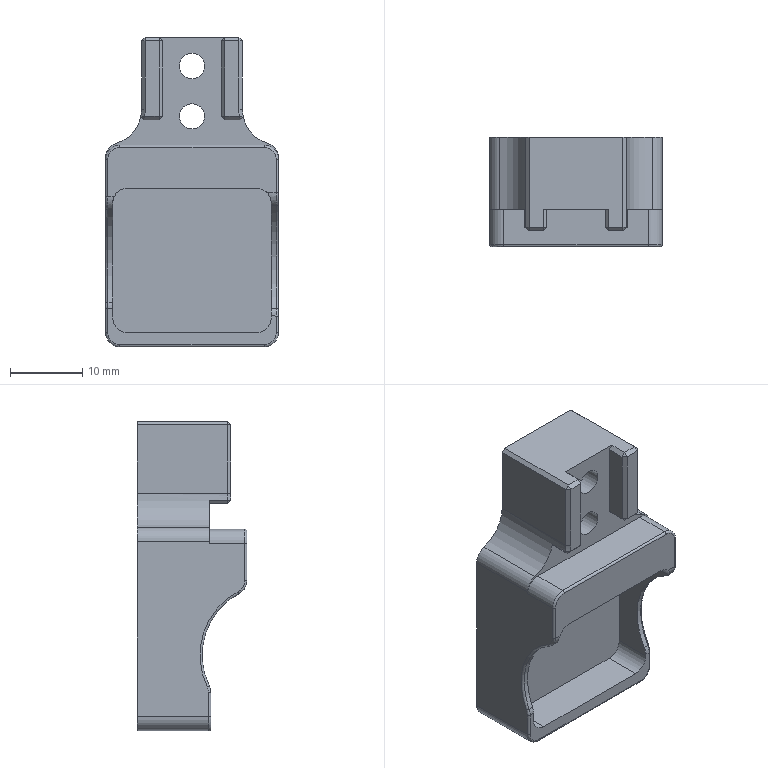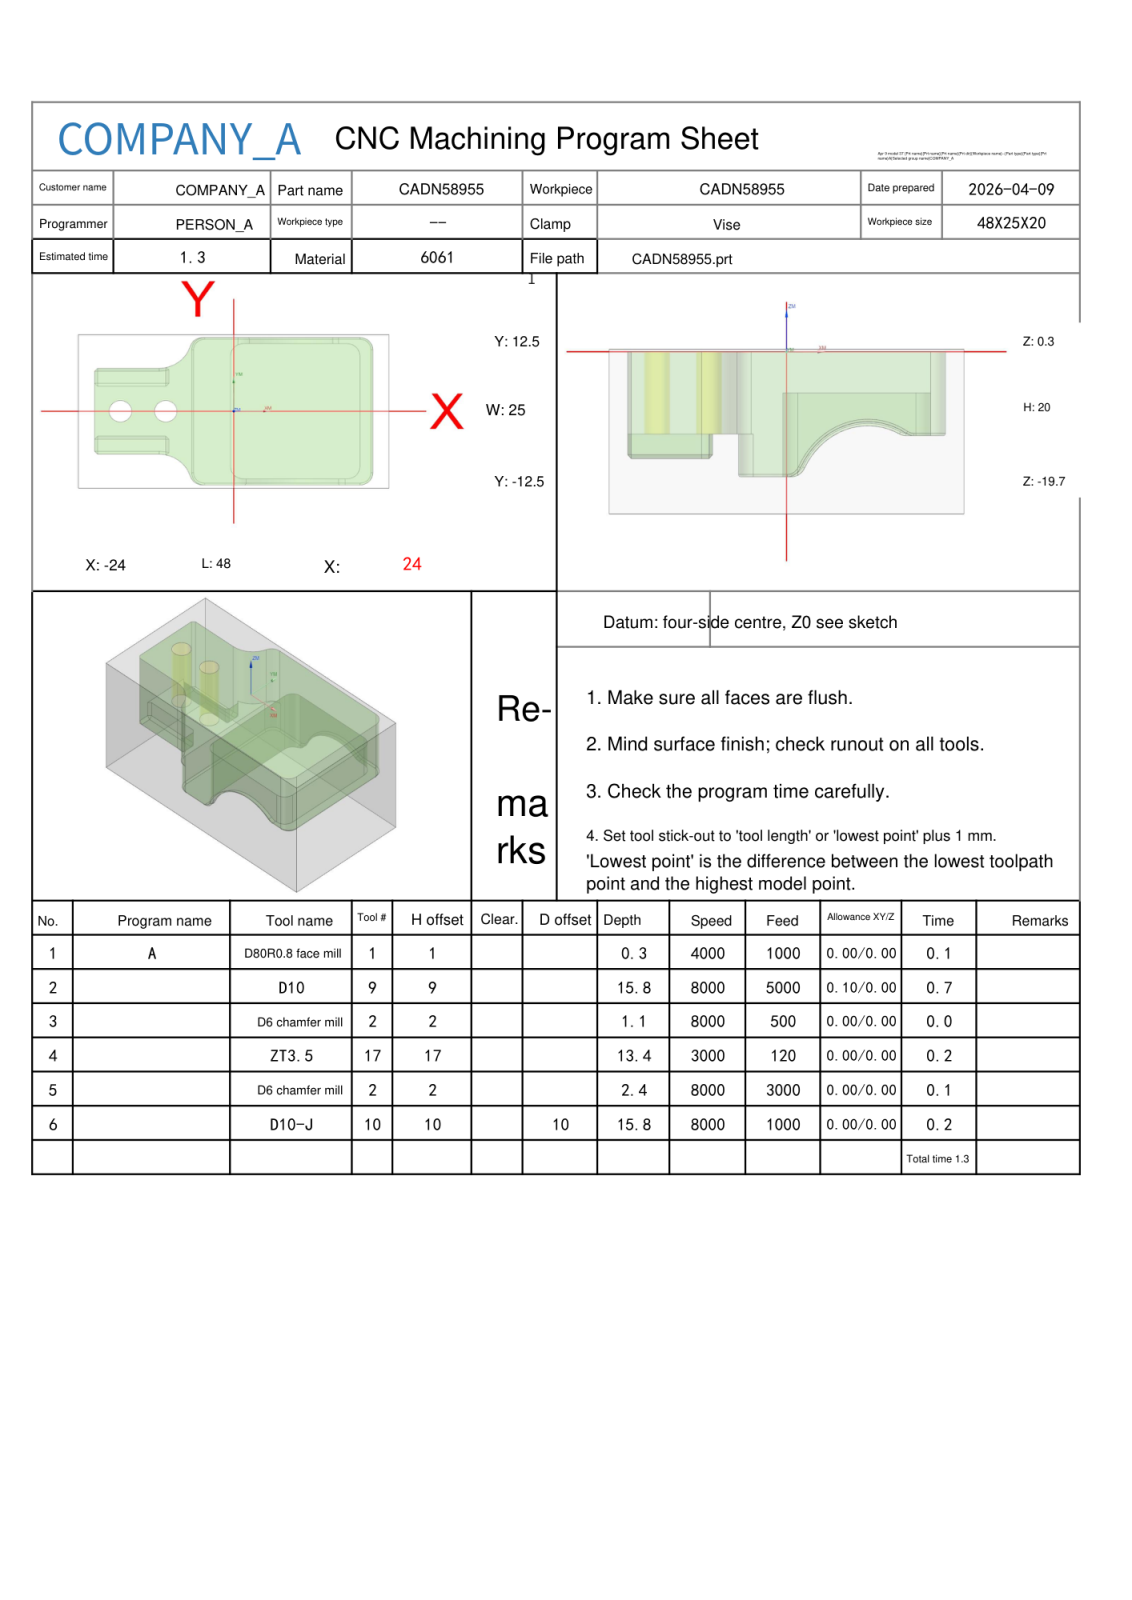NC program | NX | posted by the shop | part box 24 x 15.2 x 43 mm
Whole program:
%
O0001
(Machine time: 2.54 MIN)
(===Total Tool:5===)
(T1=D80R0.8 face mill D=80.  R=0.8  D-  H01 Z=-0.   )
(T9=D10     D=10.  R=0.   D-  H09 Z=-15.5 )
(T2=D6 chamfer mill   D=6.   R=0.   D-  H02 Z=-2.05 )
(T17=ZT3.5  D=3.5  DR_a=118 D-  H17 Z=-13.05)
(T10=D10-J  D=10.  R=0.   D10 H10 Z=-15.5 )
G80 G90 G17 G49 G40
G91 G28 Z0
M01
N1 T01 M06
(D80R0.8 face mill D=80. R=0.8 H=01 ce=0.00 di=0.00)
G00 G90 G54 X-66.5 Y0.0 M03 S4000
G43 H01 Z20.
M08
Z2.
G01 Z0.0 F1000.
X-61.5
X61.5
X66.5
Z2.
G00 Z20.
G91 G28 Z0.0
M05
M09
G91 G28 Z0.0
M01
N2 T09 M06
(D10  D=10. R=0. H=09 ce=0.10 di=0.00)
G00 G90 G54 X7.354 Y-17.1 M03 S8000
G43 H09 Z20.
M08
Z.5
G01 X-4.792 Z.442 F5000.
G02 X-11.574 Y-12.1 Z.398 I0.0 J7.1
G01 X-21. Z.353
G02 X-24.606 Y-10.606 Z.333 I0.0 J5.1
G01 X-25.106 Y-10.106 Z.33
G02 X-26.6 Y-6.5 Z.311 I3.606 J3.606
G01 Y6.5 Z.248
G02 X-25.106 Y10.106 Z.229 I5.1 J0.0
G01 X-24.606 Y10.606 Z.225
G02 X-21. Y12.1 Z.206 I3.606 J-3.606
G01 X-11.574 Z.161
G02 X-4.792 Y17.1 Z.117 I6.782 J-2.1
G01 X19.5 Z0.0
G02 X26.6 Y10. Z-.053 I0.0 J-7.1
G01 Y-10. Z-.15
G02 X19.5 Y-17.1 Z-.203 I-7.1 J0.0
G01 X-4.792 Z-.32
G02 X-11.574 Y-12.1 Z-.364 I0.0 J7.1
G01 X-21. Z-.409
G02 X-24.606 Y-10.606 Z-.429 I0.0 J5.1
G01 X-25.106 Y-10.106 Z-.432
G02 X-26.6 Y-6.5 Z-.451 I3.606 J3.606
G01 Y6.5 Z-.514
G02 X-25.106 Y10.106 Z-.533 I5.1 J0.0
G01 X-24.606 Y10.606 Z-.537
G02 X-21. Y12.1 Z-.556 I3.606 J-3.606
G01 X-11.574 Z-.601
G02 X-4.792 Y17.1 Z-.645 I6.782 J-2.1
G01 X19.5 Z-.762
G02 X26.6 Y10. Z-.815 I0.0 J-7.1
G01 Y-10. Z-.912
G02 X19.5 Y-17.1 Z-.965 I-7.1 J0.0
G01 X-4.792 Z-1.082
G02 X-11.574 Y-12.1 Z-1.126 I0.0 J7.1
G01 X-21. Z-1.171
G02 X-24.606 Y-10.606 Z-1.19 I0.0 J5.1
G01 X-25.106 Y-10.106 Z-1.194
G02 X-26.6 Y-6.5 Z-1.213 I3.606 J3.606
G01 Y6.5 Z-1.276
G02 X-25.106 Y10.106 Z-1.295 I5.1 J0.0
G01 X-24.606 Y10.606 Z-1.298
G02 X-21. Y12.1 Z-1.318 I3.606 J-3.606
G01 X-11.574 Z-1.363
G02 X-4.792 Y17.1 Z-1.407 I6.782 J-2.1
G01 X19.5 Z-1.524
G02 X26.6 Y10. Z-1.577 I0.0 J-7.1
G01 Y-10. Z-1.674
G02 X19.5 Y-17.1 Z-1.727 I-7.1 J0.0
G01 X-4.792 Z-1.844
G02 X-11.574 Y-12.1 Z-1.888 I0.0 J7.1
G01 X-21. Z-1.933
G02 X-24.606 Y-10.606 Z-1.952 I0.0 J5.1
G01 X-25.106 Y-10.106 Z-1.956
G02 X-26.6 Y-6.5 Z-1.975 I3.606 J3.606
G01 Y6.5 Z-2.038
G02 X-25.106 Y10.106 Z-2.057 I5.1 J0.0
G01 X-24.606 Y10.606 Z-2.06
G02 X-21. Y12.1 Z-2.08 I3.606 J-3.606
G01 X-11.574 Z-2.125
G02 X-4.792 Y17.1 Z-2.168 I6.782 J-2.1
G01 X19.5 Z-2.285
G02 X26.6 Y10. Z-2.339 I0.0 J-7.1
G01 Y-10. Z-2.435
G02 X19.5 Y-17.1 Z-2.489 I-7.1 J0.0
G01 X-4.792 Z-2.606
G02 X-11.574 Y-12.1 Z-2.65 I0.0 J7.1
G01 X-21. Z-2.695
G02 X-24.606 Y-10.606 Z-2.714 I0.0 J5.1
G01 X-25.106 Y-10.106 Z-2.718
G02 X-26.6 Y-6.5 Z-2.737 I3.606 J3.606
G01 Y6.5 Z-2.8
G02 X-25.106 Y10.106 Z-2.819 I5.1 J0.0
G01 X-24.606 Y10.606 Z-2.822
G02 X-21. Y12.1 Z-2.842 I3.606 J-3.606
G01 X-11.574 Z-2.887
G02 X-4.792 Y17.1 Z-2.93 I6.782 J-2.1
G01 X19.5 Z-3.047
G02 X26.6 Y10. Z-3.101 I0.0 J-7.1
G01 Y-10. Z-3.197
G02 X19.5 Y-17.1 Z-3.251 I-7.1 J0.0
G01 X-4.792 Z-3.368
G02 X-11.574 Y-12.1 Z-3.411 I0.0 J7.1
G01 X-21. Z-3.457
G02 X-24.606 Y-10.606 Z-3.476 I0.0 J5.1
G01 X-25.106 Y-10.106 Z-3.48
G02 X-26.6 Y-6.5 Z-3.499 I3.606 J3.606
G01 Y6.5 Z-3.561
G02 X-25.106 Y10.106 Z-3.581 I5.1 J0.0
G01 X-24.606 Y10.606 Z-3.584
G02 X-21. Y12.1 Z-3.603 I3.606 J-3.606
G01 X-11.574 Z-3.649
G02 X-4.792 Y17.1 Z-3.692 I6.782 J-2.1
G01 X19.5 Z-3.809
G02 X26.6 Y10. Z-3.863 I0.0 J-7.1
G01 Y-10. Z-3.959
G02 X19.5 Y-17.1 Z-4.013 I-7.1 J0.0
G01 X-4.792 Z-4.13
G02 X-11.574 Y-12.1 Z-4.173 I0.0 J7.1
G01 X-21. Z-4.219
G02 X-24.606 Y-10.606 Z-4.238 I0.0 J5.1
G01 X-25.106 Y-10.106 Z-4.241
G02 X-26.6 Y-6.5 Z-4.261 I3.606 J3.606
G01 Y6.5 Z-4.323
G02 X-25.106 Y10.106 Z-4.343 I5.1 J0.0
G01 X-24.606 Y10.606 Z-4.346
G02 X-21. Y12.1 Z-4.365 I3.606 J-3.606
G01 X-11.574 Z-4.411
G02 X-4.792 Y17.1 Z-4.454 I6.782 J-2.1
G01 X19.5 Z-4.571
G02 X26.6 Y10. Z-4.625 I0.0 J-7.1
G01 Y-10. Z-4.721
G02 X19.5 Y-17.1 Z-4.775 I-7.1 J0.0
G01 X-4.792 Z-4.892
G02 X-11.574 Y-12.1 Z-4.935 I0.0 J7.1
G01 X-21. Z-4.981
G02 X-24.606 Y-10.606 Z-5. I0.0 J5.1
G01 X-25.106 Y-10.106 Z-5.003
G02 X-26.6 Y-6.5 Z-5.023 I3.606 J3.606
G01 Y6.5 Z-5.085
G02 X-25.106 Y10.106 Z-5.105 I5.1 J0.0
G01 X-24.606 Y10.606 Z-5.108
G02 X-21. Y12.1 Z-5.127 I3.606 J-3.606
G01 X-11.574 Z-5.173
G02 X-4.792 Y17.1 Z-5.216 I6.782 J-2.1
G01 X19.5 Z-5.333
G02 X26.6 Y10. Z-5.387 I0.0 J-7.1
G01 Y-10. Z-5.483
G02 X19.5 Y-17.1 Z-5.537 I-7.1 J0.0
G01 X-4.792 Z-5.654
G02 X-11.574 Y-12.1 Z-5.697 I0.0 J7.1
G01 X-21. Z-5.743
G02 X-24.606 Y-10.606 Z-5.762 I0.0 J5.1
G01 X-25.106 Y-10.106 Z-5.765
G02 X-26.6 Y-6.5 Z-5.785 I3.606 J3.606
G01 Y6.5 Z-5.847
G02 X-25.106 Y10.106 Z-5.866 I5.1 J0.0
G01 X-24.606 Y10.606 Z-5.87
G02 X-21. Y12.1 Z-5.889 I3.606 J-3.606
G01 X-11.574 Z-5.935
G02 X-4.792 Y17.1 Z-5.978 I6.782 J-2.1
G01 X19.5 Z-6.095
G02 X26.6 Y10. Z-6.149 I0.0 J-7.1
G01 Y-10. Z-6.245
G02 X19.5 Y-17.1 Z-6.299 I-7.1 J0.0
G01 X-4.792 Z-6.416
G02 X-11.574 Y-12.1 Z-6.459 I0.0 J7.1
G01 X-21. Z-6.504
G02 X-24.606 Y-10.606 Z-6.524 I0.0 J5.1
G01 X-25.106 Y-10.106 Z-6.527
G02 X-26.6 Y-6.5 Z-6.546 I3.606 J3.606
G01 Y6.5 Z-6.609
G02 X-25.106 Y10.106 Z-6.628 I5.1 J0.0
G01 X-24.606 Y10.606 Z-6.632
G02 X-21. Y12.1 Z-6.651 I3.606 J-3.606
G01 X-11.574 Z-6.696
G02 X-4.792 Y17.1 Z-6.74 I6.782 J-2.1
G01 X19.5 Z-6.857
G02 X26.6 Y10. Z-6.911 I0.0 J-7.1
G01 Y-10. Z-7.007
G02 X19.5 Y-17.1 Z-7.061 I-7.1 J0.0
G01 X-4.792 Z-7.178
G02 X-11.574 Y-12.1 Z-7.221 I0.0 J7.1
G01 X-21. Z-7.266
G02 X-24.606 Y-10.606 Z-7.286 I0.0 J5.1
G01 X-25.106 Y-10.106 Z-7.289
G02 X-26.6 Y-6.5 Z-7.308 I3.606 J3.606
G01 Y6.5 Z-7.371
G02 X-25.106 Y10.106 Z-7.39 I5.1 J0.0
G01 X-24.606 Y10.606 Z-7.394
G02 X-21. Y12.1 Z-7.413 I3.606 J-3.606
G01 X-11.574 Z-7.458
G02 X-4.792 Y17.1 Z-7.502 I6.782 J-2.1
G01 X19.5 Z-7.619
G02 X26.6 Y10. Z-7.672 I0.0 J-7.1
G01 Y-10. Z-7.769
G02 X19.5 Y-17.1 Z-7.822 I-7.1 J0.0
G01 X-4.792 Z-7.939
G02 X-11.574 Y-12.1 Z-7.983 I0.0 J7.1
G01 X-21. Z-8.028
G02 X-24.606 Y-10.606 Z-8.048 I0.0 J5.1
G01 X-25.106 Y-10.106 Z-8.051
G02 X-26.6 Y-6.5 Z-8.07 I3.606 J3.606
G01 Y6.5 Z-8.133
G02 X-25.106 Y10.106 Z-8.152 I5.1 J0.0
G01 X-24.606 Y10.606 Z-8.156
G02 X-21. Y12.1 Z-8.175 I3.606 J-3.606
G01 X-11.574 Z-8.22
G02 X-4.792 Y17.1 Z-8.264 I6.782 J-2.1
G01 X19.5 Z-8.381
G02 X26.6 Y10. Z-8.434 I0.0 J-7.1
G01 Y-10. Z-8.531
G02 X19.5 Y-17.1 Z-8.584 I-7.1 J0.0
G01 X-4.792 Z-8.701
G02 X-11.574 Y-12.1 Z-8.745 I0.0 J7.1
G01 X-21. Z-8.79
G02 X-24.606 Y-10.606 Z-8.809 I0.0 J5.1
G01 X-25.106 Y-10.106 Z-8.813
G02 X-26.6 Y-6.5 Z-8.832 I3.606 J3.606
G01 Y6.5 Z-8.895
G02 X-25.106 Y10.106 Z-8.914 I5.1 J0.0
G01 X-24.606 Y10.606 Z-8.917
G02 X-21. Y12.1 Z-8.937 I3.606 J-3.606
G01 X-11.574 Z-8.982
G02 X-4.792 Y17.1 Z-9.026 I6.782 J-2.1
G01 X19.5 Z-9.143
G02 X26.6 Y10. Z-9.196 I0.0 J-7.1
G01 Y-10. Z-9.293
G02 X19.5 Y-17.1 Z-9.346 I-7.1 J0.0
G01 X-4.792 Z-9.463
G02 X-11.574 Y-12.1 Z-9.507 I0.0 J7.1
G01 X-21. Z-9.552
G02 X-24.606 Y-10.606 Z-9.571 I0.0 J5.1
G01 X-25.106 Y-10.106 Z-9.575
G02 X-26.6 Y-6.5 Z-9.594 I3.606 J3.606
G01 Y6.5 Z-9.657
G02 X-25.106 Y10.106 Z-9.676 I5.1 J0.0
G01 X-24.606 Y10.606 Z-9.679
G02 X-21. Y12.1 Z-9.699 I3.606 J-3.606
G01 X-11.574 Z-9.744
G02 X-4.792 Y17.1 Z-9.787 I6.782 J-2.1
G01 X19.5 Z-9.904
G02 X26.6 Y10. Z-9.958 I0.0 J-7.1
G01 Y-10. Z-10.054
G02 X19.5 Y-17.1 Z-10.108 I-7.1 J0.0
G01 X-4.792 Z-10.225
G02 X-11.574 Y-12.1 Z-10.269 I0.0 J7.1
G01 X-21. Z-10.314
G02 X-24.606 Y-10.606 Z-10.333 I0.0 J5.1
G01 X-25.106 Y-10.106 Z-10.337
G02 X-26.6 Y-6.5 Z-10.356 I3.606 J3.606
G01 Y6.5 Z-10.419
G02 X-25.106 Y10.106 Z-10.438 I5.1 J0.0
G01 X-24.606 Y10.606 Z-10.441
G02 X-21. Y12.1 Z-10.461 I3.606 J-3.606
G01 X-11.574 Z-10.506
G02 X-4.792 Y17.1 Z-10.549 I6.782 J-2.1
G01 X19.5 Z-10.666
G02 X26.6 Y10. Z-10.72 I0.0 J-7.1
G01 Y-10. Z-10.816
G02 X19.5 Y-17.1 Z-10.87 I-7.1 J0.0
G01 X-4.792 Z-10.987
G02 X-11.574 Y-12.1 Z-11.031 I0.0 J7.1
G01 X-21. Z-11.076
G02 X-24.606 Y-10.606 Z-11.095 I0.0 J5.1
G01 X-25.106 Y-10.106 Z-11.099
G02 X-26.6 Y-6.5 Z-11.118 I3.606 J3.606
G01 Y6.5 Z-11.18
G02 X-25.106 Y10.106 Z-11.2 I5.1 J0.0
G01 X-24.606 Y10.606 Z-11.203
G02 X-21. Y12.1 Z-11.222 I3.606 J-3.606
G01 X-11.574 Z-11.268
G02 X-4.792 Y17.1 Z-11.311 I6.782 J-2.1
G01 X19.5 Z-11.428
G02 X26.6 Y10. Z-11.482 I0.0 J-7.1
G01 Y-10. Z-11.578
G02 X19.5 Y-17.1 Z-11.632 I-7.1 J0.0
G01 X-4.792 Z-11.749
G02 X-11.574 Y-12.1 Z-11.792 I0.0 J7.1
G01 X-21. Z-11.838
G02 X-24.606 Y-10.606 Z-11.857 I0.0 J5.1
G01 X-25.106 Y-10.106 Z-11.86
G02 X-26.6 Y-6.5 Z-11.88 I3.606 J3.606
G01 Y6.5 Z-11.942
G02 X-25.106 Y10.106 Z-11.962 I5.1 J0.0
G01 X-24.606 Y10.606 Z-11.965
G02 X-21. Y12.1 Z-11.984 I3.606 J-3.606
G01 X-11.574 Z-12.03
G02 X-4.792 Y17.1 Z-12.073 I6.782 J-2.1
G01 X19.5 Z-12.19
G02 X26.6 Y10. Z-12.244 I0.0 J-7.1
G01 Y-10. Z-12.34
G02 X19.5 Y-17.1 Z-12.394 I-7.1 J0.0
G01 X-4.792 Z-12.511
G02 X-11.574 Y-12.1 Z-12.554 I0.0 J7.1
G01 X-21. Z-12.6
G02 X-24.606 Y-10.606 Z-12.619 I0.0 J5.1
G01 X-25.106 Y-10.106 Z-12.622
G02 X-26.6 Y-6.5 Z-12.642 I3.606 J3.606
G01 Y6.5 Z-12.704
G02 X-25.106 Y10.106 Z-12.724 I5.1 J0.0
G01 X-24.606 Y10.606 Z-12.727
G02 X-21. Y12.1 Z-12.746 I3.606 J-3.606
G01 X-11.574 Z-12.792
G02 X-4.792 Y17.1 Z-12.835 I6.782 J-2.1
G01 X19.5 Z-12.952
G02 X26.6 Y10. Z-13.006 I0.0 J-7.1
G01 Y-10. Z-13.102
G02 X19.5 Y-17.1 Z-13.156 I-7.1 J0.0
G01 X-4.792 Z-13.273
G02 X-11.574 Y-12.1 Z-13.316 I0.0 J7.1
G01 X-21. Z-13.362
G02 X-24.606 Y-10.606 Z-13.381 I0.0 J5.1
G01 X-25.106 Y-10.106 Z-13.384
G02 X-26.6 Y-6.5 Z-13.404 I3.606 J3.606
G01 Y6.5 Z-13.466
G02 X-25.106 Y10.106 Z-13.485 I5.1 J0.0
G01 X-24.606 Y10.606 Z-13.489
G02 X-21. Y12.1 Z-13.508 I3.606 J-3.606
G01 X-11.574 Z-13.554
G02 X-4.792 Y17.1 Z-13.597 I6.782 J-2.1
G01 X19.5 Z-13.714
G02 X26.6 Y10. Z-13.768 I0.0 J-7.1
G01 Y-10. Z-13.864
G02 X19.5 Y-17.1 Z-13.918 I-7.1 J0.0
G01 X-4.792 Z-14.035
G02 X-11.574 Y-12.1 Z-14.078 I0.0 J7.1
G01 X-21. Z-14.124
G02 X-24.606 Y-10.606 Z-14.143 I0.0 J5.1
G01 X-25.106 Y-10.106 Z-14.146
G02 X-26.6 Y-6.5 Z-14.165 I3.606 J3.606
G01 Y6.5 Z-14.228
G02 X-25.106 Y10.106 Z-14.247 I5.1 J0.0
G01 X-24.606 Y10.606 Z-14.251
G02 X-21. Y12.1 Z-14.27 I3.606 J-3.606
G01 X-11.574 Z-14.315
G02 X-4.792 Y17.1 Z-14.359 I6.782 J-2.1
G01 X19.5 Z-14.476
G02 X26.6 Y10. Z-14.53 I0.0 J-7.1
G01 Y-10. Z-14.626
G02 X19.5 Y-17.1 Z-14.68 I-7.1 J0.0
G01 X-4.792 Z-14.797
G02 X-11.574 Y-12.1 Z-14.84 I0.0 J7.1
G01 X-21. Z-14.885
G02 X-24.606 Y-10.606 Z-14.905 I0.0 J5.1
G01 X-25.106 Y-10.106 Z-14.908
G02 X-26.6 Y-6.5 Z-14.927 I3.606 J3.606
G01 Y6.5 Z-14.99
G02 X-25.106 Y10.106 Z-15.009 I5.1 J0.0
G01 X-24.606 Y10.606 Z-15.013
G02 X-21. Y12.1 Z-15.032 I3.606 J-3.606
G01 X-11.574 Z-15.077
G02 X-4.792 Y17.1 Z-15.121 I6.782 J-2.1
G01 X19.5 Z-15.238
G02 X26.6 Y10. Z-15.291 I0.0 J-7.1
G01 Y-10. Z-15.388
G02 X19.5 Y-17.1 Z-15.442 I-7.1 J0.0
G01 X7.354 Z-15.5
X-4.792
G02 X-11.574 Y-12.1 I0.0 J7.1
G01 X-21.
G02 X-24.606 Y-10.606 I0.0 J5.1
G01 X-25.106 Y-10.106
G02 X-26.6 Y-6.5 I3.606 J3.606
G01 Y6.5
G02 X-25.106 Y10.106 I5.1 J0.0
G01 X-24.606 Y10.606
G02 X-21. Y12.1 I3.606 J-3.606
G01 X-11.574
G02 X-4.792 Y17.1 I6.782 J-2.1
G01 X19.5
G02 X26.6 Y10. I0.0 J-7.1
G01 Y-10.
G02 X19.5 Y-17.1 I-7.1 J0.0
G01 X7.354
X6.854
Z-14.5
G00 Z20.
G91 G28 Z0.0
M05
M09
G91 G28 Z0.0
M01
N3 T02 M06
(D6 chamfer mill D=6. R=0. H=02 ce=0.00 di=0.00)
G00 G90 G54 X-10.5 Y0.0 M03 S8000
G43 H02 Z20.
M08
G98 G81 X-10.5 Y0.0 Z-.8 R1. F500.
X-17.5
G80
G00 Z20.
G91 G28 Z0.0
M05
M09
G91 G28 Z0.0
M01
N4 T17 M06
(ZT3.5 D=3.5 DR_a=118 H=17)
G00 G90 G54 X-10.5 Y0.0 M03 S3000
G43 H17 Z20.
M08
G98 G83 X-10.5 Y0.0 Z-13.052 R1. F120. Q3.
X-17.5
G80
G00 Z20.
G91 G28 Z0.0
M05
M09
G91 G28 Z0.0
M01
N5 T02 M06
(D6 chamfer mill D=6. R=0. H=02 ce=0.00 di=0.00)
G00 G90 G54 X7.104 Y13.828 M03 S8000
G43 H02 Z20.
M08
Z2.399
G01 Z-1.5 F3000.
G03 X7.024 Y13.528 I.52 J-.3
X7.324 Y13.008 I.6 J0.0
G01 X7.354 Y13.
X19.5
G02 X22.5 Y10. I0.0 J-3.
G01 Y-10.
G02 X19.5 Y-13. I-3. J0.0
G01 X-4.792
G02 X-7.667 Y-10.857 I0.0 J3.
G03 X-11.5 Y-8. I-3.833 J-1.143
G01 X-21.
X-21.259 Y-7.966
X-21.5 Y-7.866
X-21.707 Y-7.707
X-22.207 Y-7.207
X-22.366 Y-7.
X-22.466 Y-6.759
X-22.5 Y-6.5
Y6.5
X-22.466 Y6.759
X-22.366 Y7.
X-22.207 Y7.207
X-21.707 Y7.707
X-21.5 Y7.866
X-21.259 Y7.966
X-21. Y8.
X-11.5
G03 X-7.667 Y10.857 I0.0 J4.
G02 X-4.792 Y13. I2.875 J-.857
G01 X7.354
X7.384 Y13.008
G03 X7.684 Y13.528 I-.3 J.52
X7.604 Y13.828 I-.6 J0.0
G01 Z2.399
G00 Z20.
G00 G90 X-10.5 Y0.0 M03 S8000
Z20.
G98 G81 X-10.5 Y0.0 Z-2.05 R3. F500.
X-17.5
G80
G00 Z20.
G91 G28 Z0.0
M05
M09
G91 G28 Z0.0
M01
N6 T10 M06
(D10-J  D=10. R=0. H=10 ce=0.00 di=0.00)
G00 G90 G54 X-5.802 Y18.137 M03 S8000
G43 H10 Z20.
M08
Z-15.
G01 Z-15.5 F1000.
G41 D10
X-5.79 Y17.938
G03 X-4.792 Y17. I.998 J.063
G01 X19.5
G02 X26.5 Y10. I0.0 J-7.
G01 Y-10.
G02 X19.5 Y-17. I-7. J0.0
G01 X-4.792
G02 X-11.5 Y-12. I0.0 J7.
G01 X-21.
G02 X-24.536 Y-10.536 I0.0 J5.
G01 X-25.036 Y-10.036
G02 X-26.5 Y-6.5 I3.536 J3.536
G01 Y6.5
G02 X-25.036 Y10.036 I5. J0.0
G01 X-24.536 Y10.536
G02 X-21. Y12. I3.536 J-3.536
G01 X-11.5
G02 X-4.792 Y17. I6.708 J-2.
G01 X-4.292
G03 X-3.292 Y18. I0.0 J1.
G01 G40 Y18.2
Z-15.
G00 Z20.
M05
M09
G91 G28 Z0.0
G91 G28 Y0.0
M30
%